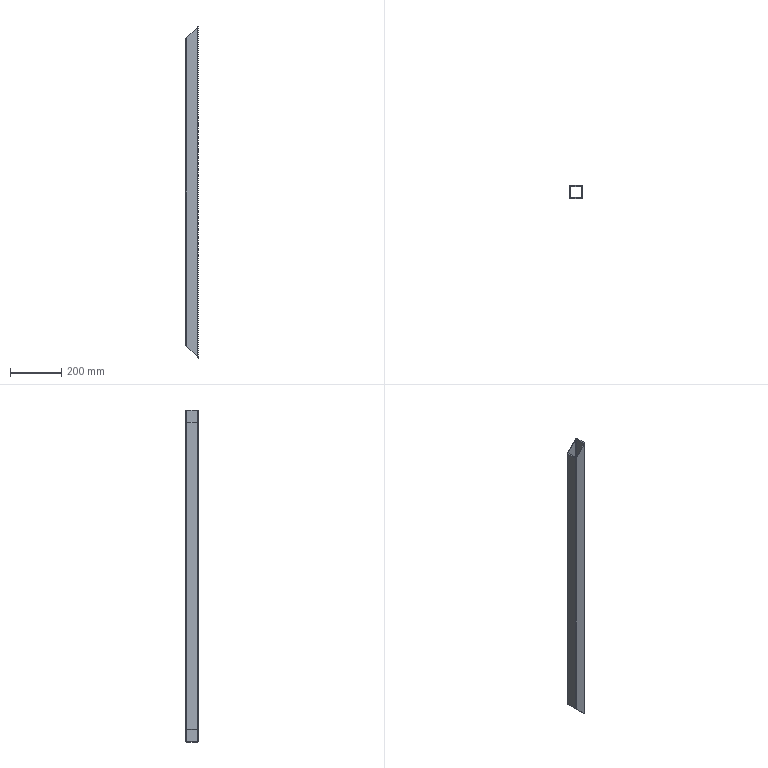Part | SolidWorks | features BaseBody 1 | 1 solid | 18 faces | box 50 x 50 x 1296 mm | volume 686700 mm3 | plane 10 | cylinder 8 | commonest cylinder face diameters 2 x4 8 x4
STEP:
#1=CARTESIAN_POINT('',(-25.,21.,598.));
#2=VERTEX_POINT('',#1);
#3=CARTESIAN_POINT('',(-25.,21.,-598.));
#4=VERTEX_POINT('',#3);
#5=CARTESIAN_POINT('',(-25.,21.,648.));
#6=DIRECTION('',(0.,0.,-1.));
#7=VECTOR('',#6,1000.);
#8=LINE('',#5,#7);
#9=EDGE_CURVE('',#2,#4,#8,.T.);
#10=ORIENTED_EDGE('',*,*,#9,.T.);
#11=CARTESIAN_POINT('',(-25.,-21.,-598.));
#12=VERTEX_POINT('',#11);
#13=CARTESIAN_POINT('',(-25.,-25.,-598.));
#14=DIRECTION('',(0.,1.,0.));
#15=VECTOR('',#14,1000.);
#16=LINE('',#13,#15);
#17=EDGE_CURVE('',#12,#4,#16,.T.);
#18=ORIENTED_EDGE('',*,*,#17,.F.);
#19=CARTESIAN_POINT('',(-25.,-21.,598.));
#20=VERTEX_POINT('',#19);
#21=CARTESIAN_POINT('',(-25.,-21.,648.));
#22=DIRECTION('',(0.,0.,-1.));
#23=VECTOR('',#22,1000.);
#24=LINE('',#21,#23);
#25=EDGE_CURVE('',#20,#12,#24,.T.);
#26=ORIENTED_EDGE('',*,*,#25,.F.);
#27=CARTESIAN_POINT('',(-25.,-25.,598.));
#28=DIRECTION('',(0.,1.,0.));
#29=VECTOR('',#28,1000.);
#30=LINE('',#27,#29);
#31=EDGE_CURVE('',#20,#2,#30,.T.);
#32=ORIENTED_EDGE('',*,*,#31,.T.);
#33=EDGE_LOOP('',(#10,#18,#26,#32));
#34=FACE_OUTER_BOUND('',#33,.T.);
#35=CARTESIAN_POINT('',(-25.,21.,648.));
#36=DIRECTION('',(1.,0.,0.));
#37=DIRECTION('',(0.,1.,0.));
#38=AXIS2_PLACEMENT_3D('',#35,#36,#37);
#39=PLANE('',#38);
#40=ADVANCED_FACE('',(#34),#39,.F.);
#41=CARTESIAN_POINT('',(-21.,25.,602.));
#42=VERTEX_POINT('',#41);
#43=CARTESIAN_POINT('',(-21.,25.,-602.));
#44=VERTEX_POINT('',#43);
#45=CARTESIAN_POINT('',(-21.,25.,648.));
#46=DIRECTION('',(0.,0.,-1.));
#47=VECTOR('',#46,1000.);
#48=LINE('',#45,#47);
#49=EDGE_CURVE('',#42,#44,#48,.T.);
#50=ORIENTED_EDGE('',*,*,#49,.T.);
#51=CARTESIAN_POINT('',(-21.,25.,-602.));
#52=CARTESIAN_POINT('',(-23.343,25.,-599.657));
#53=CARTESIAN_POINT('',(-25.,23.343,-598.));
#54=CARTESIAN_POINT('',(-25.,21.,-598.));
#55=(BOUNDED_CURVE()B_SPLINE_CURVE(3,(#51,#52,#53,#54),.UNSPECIFIED.,.F.,.F.)B_SPLINE_CURVE_WITH_KNOTS((4,4),(1.571,3.142),.UNSPECIFIED.)CURVE()GEOMETRIC_REPRESENTATION_ITEM()RATIONAL_B_SPLINE_CURVE((1.,0.8047,0.8047,1.))REPRESENTATION_ITEM(''));
#56=EDGE_CURVE('',#44,#4,#55,.T.);
#57=ORIENTED_EDGE('',*,*,#56,.T.);
#58=ORIENTED_EDGE('',*,*,#9,.F.);
#59=CARTESIAN_POINT('',(-25.,21.,598.));
#60=CARTESIAN_POINT('',(-25.,23.343,598.));
#61=CARTESIAN_POINT('',(-23.343,25.,599.657));
#62=CARTESIAN_POINT('',(-21.,25.,602.));
#63=(BOUNDED_CURVE()B_SPLINE_CURVE(3,(#59,#60,#61,#62),.UNSPECIFIED.,.F.,.F.)B_SPLINE_CURVE_WITH_KNOTS((4,4),(0.,1.571),.UNSPECIFIED.)CURVE()GEOMETRIC_REPRESENTATION_ITEM()RATIONAL_B_SPLINE_CURVE((1.,0.8047,0.8047,1.))REPRESENTATION_ITEM(''));
#64=EDGE_CURVE('',#2,#42,#63,.T.);
#65=ORIENTED_EDGE('',*,*,#64,.T.);
#66=EDGE_LOOP('',(#50,#57,#58,#65));
#67=FACE_OUTER_BOUND('',#66,.T.);
#68=CARTESIAN_POINT('',(-21.,21.,648.));
#69=DIRECTION('',(0.,0.,-1.));
#70=DIRECTION('',(-1.,0.,0.));
#71=AXIS2_PLACEMENT_3D('',#68,#69,#70);
#72=CYLINDRICAL_SURFACE('',#71,4.);
#73=ADVANCED_FACE('',(#67),#72,.T.);
#74=CARTESIAN_POINT('',(21.,25.,644.));
#75=VERTEX_POINT('',#74);
#76=CARTESIAN_POINT('',(21.,25.,-644.));
#77=VERTEX_POINT('',#76);
#78=CARTESIAN_POINT('',(21.,25.,648.));
#79=DIRECTION('',(0.,0.,-1.));
#80=VECTOR('',#79,1000.);
#81=LINE('',#78,#80);
#82=EDGE_CURVE('',#75,#77,#81,.T.);
#83=ORIENTED_EDGE('',*,*,#82,.T.);
#84=CARTESIAN_POINT('',(25.,25.,-648.));
#85=DIRECTION('',(0.7071,0.,-0.7071));
#86=VECTOR('',#85,1000.);
#87=LINE('',#84,#86);
#88=EDGE_CURVE('',#44,#77,#87,.T.);
#89=ORIENTED_EDGE('',*,*,#88,.F.);
#90=ORIENTED_EDGE('',*,*,#49,.F.);
#91=CARTESIAN_POINT('',(25.,25.,648.));
#92=DIRECTION('',(-0.7071,0.,-0.7071));
#93=VECTOR('',#92,1000.);
#94=LINE('',#91,#93);
#95=EDGE_CURVE('',#75,#42,#94,.T.);
#96=ORIENTED_EDGE('',*,*,#95,.F.);
#97=EDGE_LOOP('',(#83,#89,#90,#96));
#98=FACE_OUTER_BOUND('',#97,.T.);
#99=CARTESIAN_POINT('',(-21.,25.,648.));
#100=DIRECTION('',(0.,-1.,0.));
#101=DIRECTION('',(0.,0.,-1.));
#102=AXIS2_PLACEMENT_3D('',#99,#100,#101);
#103=PLANE('',#102);
#104=ADVANCED_FACE('',(#98),#103,.F.);
#105=CARTESIAN_POINT('',(25.,21.,648.));
#106=VERTEX_POINT('',#105);
#107=CARTESIAN_POINT('',(25.,21.,-648.));
#108=VERTEX_POINT('',#107);
#109=CARTESIAN_POINT('',(25.,21.,648.));
#110=DIRECTION('',(0.,0.,-1.));
#111=VECTOR('',#110,1000.);
#112=LINE('',#109,#111);
#113=EDGE_CURVE('',#106,#108,#112,.T.);
#114=ORIENTED_EDGE('',*,*,#113,.T.);
#115=CARTESIAN_POINT('',(25.,21.,-648.));
#116=CARTESIAN_POINT('',(25.,23.343,-648.));
#117=CARTESIAN_POINT('',(23.343,25.,-646.343));
#118=CARTESIAN_POINT('',(21.,25.,-644.));
#119=(BOUNDED_CURVE()B_SPLINE_CURVE(3,(#115,#116,#117,#118),.UNSPECIFIED.,.F.,.F.)B_SPLINE_CURVE_WITH_KNOTS((4,4),(0.,1.571),.UNSPECIFIED.)CURVE()GEOMETRIC_REPRESENTATION_ITEM()RATIONAL_B_SPLINE_CURVE((1.,0.8047,0.8047,1.))REPRESENTATION_ITEM(''));
#120=EDGE_CURVE('',#108,#77,#119,.T.);
#121=ORIENTED_EDGE('',*,*,#120,.T.);
#122=ORIENTED_EDGE('',*,*,#82,.F.);
#123=CARTESIAN_POINT('',(21.,25.,644.));
#124=CARTESIAN_POINT('',(23.343,25.,646.343));
#125=CARTESIAN_POINT('',(25.,23.343,648.));
#126=CARTESIAN_POINT('',(25.,21.,648.));
#127=(BOUNDED_CURVE()B_SPLINE_CURVE(3,(#123,#124,#125,#126),.UNSPECIFIED.,.F.,.F.)B_SPLINE_CURVE_WITH_KNOTS((4,4),(1.571,3.142),.UNSPECIFIED.)CURVE()GEOMETRIC_REPRESENTATION_ITEM()RATIONAL_B_SPLINE_CURVE((1.,0.8047,0.8047,1.))REPRESENTATION_ITEM(''));
#128=EDGE_CURVE('',#75,#106,#127,.T.);
#129=ORIENTED_EDGE('',*,*,#128,.T.);
#130=EDGE_LOOP('',(#114,#121,#122,#129));
#131=FACE_OUTER_BOUND('',#130,.T.);
#132=CARTESIAN_POINT('',(21.,21.,648.));
#133=DIRECTION('',(0.,0.,-1.));
#134=DIRECTION('',(-1.,0.,0.));
#135=AXIS2_PLACEMENT_3D('',#132,#133,#134);
#136=CYLINDRICAL_SURFACE('',#135,4.);
#137=ADVANCED_FACE('',(#131),#136,.T.);
#138=CARTESIAN_POINT('',(25.,-21.,-648.));
#139=VERTEX_POINT('',#138);
#140=CARTESIAN_POINT('',(25.,21.,-648.));
#141=DIRECTION('',(0.,1.,0.));
#142=VECTOR('',#141,1000.);
#143=LINE('',#140,#142);
#144=EDGE_CURVE('',#139,#108,#143,.T.);
#145=ORIENTED_EDGE('',*,*,#144,.T.);
#146=ORIENTED_EDGE('',*,*,#113,.F.);
#147=CARTESIAN_POINT('',(25.,-21.,648.));
#148=VERTEX_POINT('',#147);
#149=CARTESIAN_POINT('',(25.,21.,648.));
#150=DIRECTION('',(0.,1.,0.));
#151=VECTOR('',#150,1000.);
#152=LINE('',#149,#151);
#153=EDGE_CURVE('',#148,#106,#152,.T.);
#154=ORIENTED_EDGE('',*,*,#153,.F.);
#155=CARTESIAN_POINT('',(25.,-21.,648.));
#156=DIRECTION('',(0.,0.,-1.));
#157=VECTOR('',#156,1000.);
#158=LINE('',#155,#157);
#159=EDGE_CURVE('',#148,#139,#158,.T.);
#160=ORIENTED_EDGE('',*,*,#159,.T.);
#161=EDGE_LOOP('',(#145,#146,#154,#160));
#162=FACE_OUTER_BOUND('',#161,.T.);
#163=CARTESIAN_POINT('',(25.,21.,648.));
#164=DIRECTION('',(-1.,0.,0.));
#165=DIRECTION('',(0.,1.,0.));
#166=AXIS2_PLACEMENT_3D('',#163,#164,#165);
#167=PLANE('',#166);
#168=ADVANCED_FACE('',(#162),#167,.F.);
#169=CARTESIAN_POINT('',(21.,-25.,644.));
#170=VERTEX_POINT('',#169);
#171=CARTESIAN_POINT('',(21.,-25.,-644.));
#172=VERTEX_POINT('',#171);
#173=CARTESIAN_POINT('',(21.,-25.,648.));
#174=DIRECTION('',(0.,0.,-1.));
#175=VECTOR('',#174,1000.);
#176=LINE('',#173,#175);
#177=EDGE_CURVE('',#170,#172,#176,.T.);
#178=ORIENTED_EDGE('',*,*,#177,.T.);
#179=CARTESIAN_POINT('',(21.,-25.,-644.));
#180=CARTESIAN_POINT('',(23.343,-25.,-646.343));
#181=CARTESIAN_POINT('',(25.,-23.343,-648.));
#182=CARTESIAN_POINT('',(25.,-21.,-648.));
#183=(BOUNDED_CURVE()B_SPLINE_CURVE(3,(#179,#180,#181,#182),.UNSPECIFIED.,.F.,.F.)B_SPLINE_CURVE_WITH_KNOTS((4,4),(4.712,6.283),.UNSPECIFIED.)CURVE()GEOMETRIC_REPRESENTATION_ITEM()RATIONAL_B_SPLINE_CURVE((1.,0.8047,0.8047,1.))REPRESENTATION_ITEM(''));
#184=EDGE_CURVE('',#172,#139,#183,.T.);
#185=ORIENTED_EDGE('',*,*,#184,.T.);
#186=ORIENTED_EDGE('',*,*,#159,.F.);
#187=CARTESIAN_POINT('',(25.,-21.,648.));
#188=CARTESIAN_POINT('',(25.,-23.343,648.));
#189=CARTESIAN_POINT('',(23.343,-25.,646.343));
#190=CARTESIAN_POINT('',(21.,-25.,644.));
#191=(BOUNDED_CURVE()B_SPLINE_CURVE(3,(#187,#188,#189,#190),.UNSPECIFIED.,.F.,.F.)B_SPLINE_CURVE_WITH_KNOTS((4,4),(3.142,4.712),.UNSPECIFIED.)CURVE()GEOMETRIC_REPRESENTATION_ITEM()RATIONAL_B_SPLINE_CURVE((1.,0.8047,0.8047,1.))REPRESENTATION_ITEM(''));
#192=EDGE_CURVE('',#148,#170,#191,.T.);
#193=ORIENTED_EDGE('',*,*,#192,.T.);
#194=EDGE_LOOP('',(#178,#185,#186,#193));
#195=FACE_OUTER_BOUND('',#194,.T.);
#196=CARTESIAN_POINT('',(21.,-21.,648.));
#197=DIRECTION('',(0.,0.,-1.));
#198=DIRECTION('',(-1.,0.,0.));
#199=AXIS2_PLACEMENT_3D('',#196,#197,#198);
#200=CYLINDRICAL_SURFACE('',#199,4.);
#201=ADVANCED_FACE('',(#195),#200,.T.);
#202=CARTESIAN_POINT('',(-21.,-25.,602.));
#203=VERTEX_POINT('',#202);
#204=CARTESIAN_POINT('',(-21.,-25.,-602.));
#205=VERTEX_POINT('',#204);
#206=CARTESIAN_POINT('',(-21.,-25.,648.));
#207=DIRECTION('',(0.,0.,-1.));
#208=VECTOR('',#207,1000.);
#209=LINE('',#206,#208);
#210=EDGE_CURVE('',#203,#205,#209,.T.);
#211=ORIENTED_EDGE('',*,*,#210,.T.);
#212=CARTESIAN_POINT('',(25.,-25.,-648.));
#213=DIRECTION('',(0.7071,0.,-0.7071));
#214=VECTOR('',#213,1000.);
#215=LINE('',#212,#214);
#216=EDGE_CURVE('',#205,#172,#215,.T.);
#217=ORIENTED_EDGE('',*,*,#216,.T.);
#218=ORIENTED_EDGE('',*,*,#177,.F.);
#219=CARTESIAN_POINT('',(25.,-25.,648.));
#220=DIRECTION('',(-0.7071,0.,-0.7071));
#221=VECTOR('',#220,1000.);
#222=LINE('',#219,#221);
#223=EDGE_CURVE('',#170,#203,#222,.T.);
#224=ORIENTED_EDGE('',*,*,#223,.T.);
#225=EDGE_LOOP('',(#211,#217,#218,#224));
#226=FACE_OUTER_BOUND('',#225,.T.);
#227=CARTESIAN_POINT('',(-21.,-25.,648.));
#228=DIRECTION('',(0.,1.,0.));
#229=DIRECTION('',(1.,0.,0.));
#230=AXIS2_PLACEMENT_3D('',#227,#228,#229);
#231=PLANE('',#230);
#232=ADVANCED_FACE('',(#226),#231,.F.);
#233=ORIENTED_EDGE('',*,*,#25,.T.);
#234=CARTESIAN_POINT('',(-25.,-21.,-598.));
#235=CARTESIAN_POINT('',(-25.,-23.343,-598.));
#236=CARTESIAN_POINT('',(-23.343,-25.,-599.657));
#237=CARTESIAN_POINT('',(-21.,-25.,-602.));
#238=(BOUNDED_CURVE()B_SPLINE_CURVE(3,(#234,#235,#236,#237),.UNSPECIFIED.,.F.,.F.)B_SPLINE_CURVE_WITH_KNOTS((4,4),(3.142,4.712),.UNSPECIFIED.)CURVE()GEOMETRIC_REPRESENTATION_ITEM()RATIONAL_B_SPLINE_CURVE((1.,0.8047,0.8047,1.))REPRESENTATION_ITEM(''));
#239=EDGE_CURVE('',#12,#205,#238,.T.);
#240=ORIENTED_EDGE('',*,*,#239,.T.);
#241=ORIENTED_EDGE('',*,*,#210,.F.);
#242=CARTESIAN_POINT('',(-21.,-25.,602.));
#243=CARTESIAN_POINT('',(-23.343,-25.,599.657));
#244=CARTESIAN_POINT('',(-25.,-23.343,598.));
#245=CARTESIAN_POINT('',(-25.,-21.,598.));
#246=(BOUNDED_CURVE()B_SPLINE_CURVE(3,(#242,#243,#244,#245),.UNSPECIFIED.,.F.,.F.)B_SPLINE_CURVE_WITH_KNOTS((4,4),(4.712,6.283),.UNSPECIFIED.)CURVE()GEOMETRIC_REPRESENTATION_ITEM()RATIONAL_B_SPLINE_CURVE((1.,0.8047,0.8047,1.))REPRESENTATION_ITEM(''));
#247=EDGE_CURVE('',#203,#20,#246,.T.);
#248=ORIENTED_EDGE('',*,*,#247,.T.);
#249=EDGE_LOOP('',(#233,#240,#241,#248));
#250=FACE_OUTER_BOUND('',#249,.T.);
#251=CARTESIAN_POINT('',(-21.,-21.,648.));
#252=DIRECTION('',(0.,0.,-1.));
#253=DIRECTION('',(-1.,0.,0.));
#254=AXIS2_PLACEMENT_3D('',#251,#252,#253);
#255=CYLINDRICAL_SURFACE('',#254,4.);
#256=ADVANCED_FACE('',(#250),#255,.T.);
#257=CARTESIAN_POINT('',(-22.,-21.,-601.));
#258=VERTEX_POINT('',#257);
#259=CARTESIAN_POINT('',(-21.,-22.,-602.));
#260=VERTEX_POINT('',#259);
#261=CARTESIAN_POINT('',(-22.,-21.,-601.));
#262=CARTESIAN_POINT('',(-22.,-21.586,-601.));
#263=CARTESIAN_POINT('',(-21.586,-22.,-601.414));
#264=CARTESIAN_POINT('',(-21.,-22.,-602.));
#265=(BOUNDED_CURVE()B_SPLINE_CURVE(3,(#261,#262,#263,#264),.UNSPECIFIED.,.F.,.F.)B_SPLINE_CURVE_WITH_KNOTS((4,4),(3.142,4.712),.UNSPECIFIED.)CURVE()GEOMETRIC_REPRESENTATION_ITEM()RATIONAL_B_SPLINE_CURVE((1.,0.8047,0.8047,1.))REPRESENTATION_ITEM(''));
#266=EDGE_CURVE('',#258,#260,#265,.T.);
#267=ORIENTED_EDGE('',*,*,#266,.T.);
#268=CARTESIAN_POINT('',(21.,-22.,-644.));
#269=VERTEX_POINT('',#268);
#270=CARTESIAN_POINT('',(-646.,-22.,23.));
#271=DIRECTION('',(0.7071,0.,-0.7071));
#272=VECTOR('',#271,1000.);
#273=LINE('',#270,#272);
#274=EDGE_CURVE('',#260,#269,#273,.T.);
#275=ORIENTED_EDGE('',*,*,#274,.T.);
#276=CARTESIAN_POINT('',(22.,-21.,-645.));
#277=VERTEX_POINT('',#276);
#278=CARTESIAN_POINT('',(21.,-22.,-644.));
#279=CARTESIAN_POINT('',(21.586,-22.,-644.586));
#280=CARTESIAN_POINT('',(22.,-21.586,-645.));
#281=CARTESIAN_POINT('',(22.,-21.,-645.));
#282=(BOUNDED_CURVE()B_SPLINE_CURVE(3,(#278,#279,#280,#281),.UNSPECIFIED.,.F.,.F.)B_SPLINE_CURVE_WITH_KNOTS((4,4),(4.712,6.283),.UNSPECIFIED.)CURVE()GEOMETRIC_REPRESENTATION_ITEM()RATIONAL_B_SPLINE_CURVE((1.,0.8047,0.8047,1.))REPRESENTATION_ITEM(''));
#283=EDGE_CURVE('',#269,#277,#282,.T.);
#284=ORIENTED_EDGE('',*,*,#283,.T.);
#285=CARTESIAN_POINT('',(22.,21.,-645.));
#286=VERTEX_POINT('',#285);
#287=CARTESIAN_POINT('',(22.,21.,-645.));
#288=DIRECTION('',(0.,1.,0.));
#289=VECTOR('',#288,1000.);
#290=LINE('',#287,#289);
#291=EDGE_CURVE('',#277,#286,#290,.T.);
#292=ORIENTED_EDGE('',*,*,#291,.T.);
#293=CARTESIAN_POINT('',(21.,22.,-644.));
#294=VERTEX_POINT('',#293);
#295=CARTESIAN_POINT('',(22.,21.,-645.));
#296=CARTESIAN_POINT('',(22.,21.586,-645.));
#297=CARTESIAN_POINT('',(21.586,22.,-644.586));
#298=CARTESIAN_POINT('',(21.,22.,-644.));
#299=(BOUNDED_CURVE()B_SPLINE_CURVE(3,(#295,#296,#297,#298),.UNSPECIFIED.,.F.,.F.)B_SPLINE_CURVE_WITH_KNOTS((4,4),(0.,1.571),.UNSPECIFIED.)CURVE()GEOMETRIC_REPRESENTATION_ITEM()RATIONAL_B_SPLINE_CURVE((1.,0.8047,0.8047,1.))REPRESENTATION_ITEM(''));
#300=EDGE_CURVE('',#286,#294,#299,.T.);
#301=ORIENTED_EDGE('',*,*,#300,.T.);
#302=CARTESIAN_POINT('',(-21.,22.,-602.));
#303=VERTEX_POINT('',#302);
#304=CARTESIAN_POINT('',(-646.,22.,23.));
#305=DIRECTION('',(-0.7071,0.,0.7071));
#306=VECTOR('',#305,1000.);
#307=LINE('',#304,#306);
#308=EDGE_CURVE('',#294,#303,#307,.T.);
#309=ORIENTED_EDGE('',*,*,#308,.T.);
#310=CARTESIAN_POINT('',(-22.,21.,-601.));
#311=VERTEX_POINT('',#310);
#312=CARTESIAN_POINT('',(-21.,22.,-602.));
#313=CARTESIAN_POINT('',(-21.586,22.,-601.414));
#314=CARTESIAN_POINT('',(-22.,21.586,-601.));
#315=CARTESIAN_POINT('',(-22.,21.,-601.));
#316=(BOUNDED_CURVE()B_SPLINE_CURVE(3,(#312,#313,#314,#315),.UNSPECIFIED.,.F.,.F.)B_SPLINE_CURVE_WITH_KNOTS((4,4),(1.571,3.142),.UNSPECIFIED.)CURVE()GEOMETRIC_REPRESENTATION_ITEM()RATIONAL_B_SPLINE_CURVE((1.,0.8047,0.8047,1.))REPRESENTATION_ITEM(''));
#317=EDGE_CURVE('',#303,#311,#316,.T.);
#318=ORIENTED_EDGE('',*,*,#317,.T.);
#319=CARTESIAN_POINT('',(-22.,21.,-601.));
#320=DIRECTION('',(0.,-1.,0.));
#321=VECTOR('',#320,1000.);
#322=LINE('',#319,#321);
#323=EDGE_CURVE('',#311,#258,#322,.T.);
#324=ORIENTED_EDGE('',*,*,#323,.T.);
#325=EDGE_LOOP('',(#267,#275,#284,#292,#301,#309,#318,#324));
#326=FACE_BOUND('',#325,.T.);
#327=ORIENTED_EDGE('',*,*,#17,.T.);
#328=ORIENTED_EDGE('',*,*,#56,.F.);
#329=ORIENTED_EDGE('',*,*,#88,.T.);
#330=ORIENTED_EDGE('',*,*,#120,.F.);
#331=ORIENTED_EDGE('',*,*,#144,.F.);
#332=ORIENTED_EDGE('',*,*,#184,.F.);
#333=ORIENTED_EDGE('',*,*,#216,.F.);
#334=ORIENTED_EDGE('',*,*,#239,.F.);
#335=EDGE_LOOP('',(#327,#328,#329,#330,#331,#332,#333,#334));
#336=FACE_OUTER_BOUND('',#335,.T.);
#337=CARTESIAN_POINT('',(25.,-25.,-648.));
#338=DIRECTION('',(0.7071,0.,0.7071));
#339=DIRECTION('',(0.,-1.,0.));
#340=AXIS2_PLACEMENT_3D('',#337,#338,#339);
#341=PLANE('',#340);
#342=ADVANCED_FACE('',(#326,#336),#341,.F.);
#343=CARTESIAN_POINT('',(-21.,-22.,602.));
#344=VERTEX_POINT('',#343);
#345=CARTESIAN_POINT('',(-22.,-21.,601.));
#346=VERTEX_POINT('',#345);
#347=CARTESIAN_POINT('',(-21.,-22.,602.));
#348=CARTESIAN_POINT('',(-21.586,-22.,601.414));
#349=CARTESIAN_POINT('',(-22.,-21.586,601.));
#350=CARTESIAN_POINT('',(-22.,-21.,601.));
#351=(BOUNDED_CURVE()B_SPLINE_CURVE(3,(#347,#348,#349,#350),.UNSPECIFIED.,.F.,.F.)B_SPLINE_CURVE_WITH_KNOTS((4,4),(4.712,6.283),.UNSPECIFIED.)CURVE()GEOMETRIC_REPRESENTATION_ITEM()RATIONAL_B_SPLINE_CURVE((1.,0.8047,0.8047,1.))REPRESENTATION_ITEM(''));
#352=EDGE_CURVE('',#344,#346,#351,.T.);
#353=ORIENTED_EDGE('',*,*,#352,.T.);
#354=CARTESIAN_POINT('',(-22.,21.,601.));
#355=VERTEX_POINT('',#354);
#356=CARTESIAN_POINT('',(-22.,21.,601.));
#357=DIRECTION('',(0.,1.,0.));
#358=VECTOR('',#357,1000.);
#359=LINE('',#356,#358);
#360=EDGE_CURVE('',#346,#355,#359,.T.);
#361=ORIENTED_EDGE('',*,*,#360,.T.);
#362=CARTESIAN_POINT('',(-21.,22.,602.));
#363=VERTEX_POINT('',#362);
#364=CARTESIAN_POINT('',(-22.,21.,601.));
#365=CARTESIAN_POINT('',(-22.,21.586,601.));
#366=CARTESIAN_POINT('',(-21.586,22.,601.414));
#367=CARTESIAN_POINT('',(-21.,22.,602.));
#368=(BOUNDED_CURVE()B_SPLINE_CURVE(3,(#364,#365,#366,#367),.UNSPECIFIED.,.F.,.F.)B_SPLINE_CURVE_WITH_KNOTS((4,4),(0.,1.571),.UNSPECIFIED.)CURVE()GEOMETRIC_REPRESENTATION_ITEM()RATIONAL_B_SPLINE_CURVE((1.,0.8047,0.8047,1.))REPRESENTATION_ITEM(''));
#369=EDGE_CURVE('',#355,#363,#368,.T.);
#370=ORIENTED_EDGE('',*,*,#369,.T.);
#371=CARTESIAN_POINT('',(21.,22.,644.));
#372=VERTEX_POINT('',#371);
#373=CARTESIAN_POINT('',(2.,22.,625.));
#374=DIRECTION('',(0.7071,0.,0.7071));
#375=VECTOR('',#374,1000.);
#376=LINE('',#373,#375);
#377=EDGE_CURVE('',#363,#372,#376,.T.);
#378=ORIENTED_EDGE('',*,*,#377,.T.);
#379=CARTESIAN_POINT('',(22.,21.,645.));
#380=VERTEX_POINT('',#379);
#381=CARTESIAN_POINT('',(21.,22.,644.));
#382=CARTESIAN_POINT('',(21.586,22.,644.586));
#383=CARTESIAN_POINT('',(22.,21.586,645.));
#384=CARTESIAN_POINT('',(22.,21.,645.));
#385=(BOUNDED_CURVE()B_SPLINE_CURVE(3,(#381,#382,#383,#384),.UNSPECIFIED.,.F.,.F.)B_SPLINE_CURVE_WITH_KNOTS((4,4),(1.571,3.142),.UNSPECIFIED.)CURVE()GEOMETRIC_REPRESENTATION_ITEM()RATIONAL_B_SPLINE_CURVE((1.,0.8047,0.8047,1.))REPRESENTATION_ITEM(''));
#386=EDGE_CURVE('',#372,#380,#385,.T.);
#387=ORIENTED_EDGE('',*,*,#386,.T.);
#388=CARTESIAN_POINT('',(22.,-21.,645.));
#389=VERTEX_POINT('',#388);
#390=CARTESIAN_POINT('',(22.,21.,645.));
#391=DIRECTION('',(0.,-1.,0.));
#392=VECTOR('',#391,1000.);
#393=LINE('',#390,#392);
#394=EDGE_CURVE('',#380,#389,#393,.T.);
#395=ORIENTED_EDGE('',*,*,#394,.T.);
#396=CARTESIAN_POINT('',(21.,-22.,644.));
#397=VERTEX_POINT('',#396);
#398=CARTESIAN_POINT('',(22.,-21.,645.));
#399=CARTESIAN_POINT('',(22.,-21.586,645.));
#400=CARTESIAN_POINT('',(21.586,-22.,644.586));
#401=CARTESIAN_POINT('',(21.,-22.,644.));
#402=(BOUNDED_CURVE()B_SPLINE_CURVE(3,(#398,#399,#400,#401),.UNSPECIFIED.,.F.,.F.)B_SPLINE_CURVE_WITH_KNOTS((4,4),(3.142,4.712),.UNSPECIFIED.)CURVE()GEOMETRIC_REPRESENTATION_ITEM()RATIONAL_B_SPLINE_CURVE((1.,0.8047,0.8047,1.))REPRESENTATION_ITEM(''));
#403=EDGE_CURVE('',#389,#397,#402,.T.);
#404=ORIENTED_EDGE('',*,*,#403,.T.);
#405=CARTESIAN_POINT('',(2.,-22.,625.));
#406=DIRECTION('',(-0.7071,0.,-0.7071));
#407=VECTOR('',#406,1000.);
#408=LINE('',#405,#407);
#409=EDGE_CURVE('',#397,#344,#408,.T.);
#410=ORIENTED_EDGE('',*,*,#409,.T.);
#411=EDGE_LOOP('',(#353,#361,#370,#378,#387,#395,#404,#410));
#412=FACE_BOUND('',#411,.T.);
#413=ORIENTED_EDGE('',*,*,#223,.F.);
#414=ORIENTED_EDGE('',*,*,#192,.F.);
#415=ORIENTED_EDGE('',*,*,#153,.T.);
#416=ORIENTED_EDGE('',*,*,#128,.F.);
#417=ORIENTED_EDGE('',*,*,#95,.T.);
#418=ORIENTED_EDGE('',*,*,#64,.F.);
#419=ORIENTED_EDGE('',*,*,#31,.F.);
#420=ORIENTED_EDGE('',*,*,#247,.F.);
#421=EDGE_LOOP('',(#413,#414,#415,#416,#417,#418,#419,#420));
#422=FACE_OUTER_BOUND('',#421,.T.);
#423=CARTESIAN_POINT('',(25.,-25.,648.));
#424=DIRECTION('',(0.7071,0.,-0.7071));
#425=DIRECTION('',(0.,-1.,0.));
#426=AXIS2_PLACEMENT_3D('',#423,#424,#425);
#427=PLANE('',#426);
#428=ADVANCED_FACE('',(#412,#422),#427,.F.);
#429=ORIENTED_EDGE('',*,*,#266,.F.);
#430=CARTESIAN_POINT('',(-22.,-21.,648.));
#431=DIRECTION('',(0.,0.,-1.));
#432=VECTOR('',#431,1000.);
#433=LINE('',#430,#432);
#434=EDGE_CURVE('',#346,#258,#433,.T.);
#435=ORIENTED_EDGE('',*,*,#434,.F.);
#436=ORIENTED_EDGE('',*,*,#352,.F.);
#437=CARTESIAN_POINT('',(-21.,-22.,648.));
#438=DIRECTION('',(0.,0.,-1.));
#439=VECTOR('',#438,1000.);
#440=LINE('',#437,#439);
#441=EDGE_CURVE('',#344,#260,#440,.T.);
#442=ORIENTED_EDGE('',*,*,#441,.T.);
#443=EDGE_LOOP('',(#429,#435,#436,#442));
#444=FACE_OUTER_BOUND('',#443,.T.);
#445=CARTESIAN_POINT('',(-21.,-21.,648.));
#446=DIRECTION('',(0.,0.,-1.));
#447=DIRECTION('',(-1.,0.,0.));
#448=AXIS2_PLACEMENT_3D('',#445,#446,#447);
#449=CYLINDRICAL_SURFACE('',#448,1.);
#450=ADVANCED_FACE('',(#444),#449,.F.);
#451=ORIENTED_EDGE('',*,*,#274,.F.);
#452=ORIENTED_EDGE('',*,*,#441,.F.);
#453=ORIENTED_EDGE('',*,*,#409,.F.);
#454=CARTESIAN_POINT('',(21.,-22.,648.));
#455=DIRECTION('',(0.,0.,-1.));
#456=VECTOR('',#455,1000.);
#457=LINE('',#454,#456);
#458=EDGE_CURVE('',#397,#269,#457,.T.);
#459=ORIENTED_EDGE('',*,*,#458,.T.);
#460=EDGE_LOOP('',(#451,#452,#453,#459));
#461=FACE_OUTER_BOUND('',#460,.T.);
#462=CARTESIAN_POINT('',(-21.,-22.,648.));
#463=DIRECTION('',(0.,1.,0.));
#464=DIRECTION('',(1.,0.,0.));
#465=AXIS2_PLACEMENT_3D('',#462,#463,#464);
#466=PLANE('',#465);
#467=ADVANCED_FACE('',(#461),#466,.T.);
#468=ORIENTED_EDGE('',*,*,#283,.F.);
#469=ORIENTED_EDGE('',*,*,#458,.F.);
#470=ORIENTED_EDGE('',*,*,#403,.F.);
#471=CARTESIAN_POINT('',(22.,-21.,648.));
#472=DIRECTION('',(0.,0.,-1.));
#473=VECTOR('',#472,1000.);
#474=LINE('',#471,#473);
#475=EDGE_CURVE('',#389,#277,#474,.T.);
#476=ORIENTED_EDGE('',*,*,#475,.T.);
#477=EDGE_LOOP('',(#468,#469,#470,#476));
#478=FACE_OUTER_BOUND('',#477,.T.);
#479=CARTESIAN_POINT('',(21.,-21.,648.));
#480=DIRECTION('',(0.,0.,-1.));
#481=DIRECTION('',(-1.,0.,0.));
#482=AXIS2_PLACEMENT_3D('',#479,#480,#481);
#483=CYLINDRICAL_SURFACE('',#482,1.);
#484=ADVANCED_FACE('',(#478),#483,.F.);
#485=ORIENTED_EDGE('',*,*,#291,.F.);
#486=ORIENTED_EDGE('',*,*,#475,.F.);
#487=ORIENTED_EDGE('',*,*,#394,.F.);
#488=CARTESIAN_POINT('',(22.,21.,648.));
#489=DIRECTION('',(0.,0.,-1.));
#490=VECTOR('',#489,1000.);
#491=LINE('',#488,#490);
#492=EDGE_CURVE('',#380,#286,#491,.T.);
#493=ORIENTED_EDGE('',*,*,#492,.T.);
#494=EDGE_LOOP('',(#485,#486,#487,#493));
#495=FACE_OUTER_BOUND('',#494,.T.);
#496=CARTESIAN_POINT('',(22.,21.,648.));
#497=DIRECTION('',(-1.,0.,0.));
#498=DIRECTION('',(0.,1.,0.));
#499=AXIS2_PLACEMENT_3D('',#496,#497,#498);
#500=PLANE('',#499);
#501=ADVANCED_FACE('',(#495),#500,.T.);
#502=ORIENTED_EDGE('',*,*,#300,.F.);
#503=ORIENTED_EDGE('',*,*,#492,.F.);
#504=ORIENTED_EDGE('',*,*,#386,.F.);
#505=CARTESIAN_POINT('',(21.,22.,648.));
#506=DIRECTION('',(0.,0.,-1.));
#507=VECTOR('',#506,1000.);
#508=LINE('',#505,#507);
#509=EDGE_CURVE('',#372,#294,#508,.T.);
#510=ORIENTED_EDGE('',*,*,#509,.T.);
#511=EDGE_LOOP('',(#502,#503,#504,#510));
#512=FACE_OUTER_BOUND('',#511,.T.);
#513=CARTESIAN_POINT('',(21.,21.,648.));
#514=DIRECTION('',(0.,0.,-1.));
#515=DIRECTION('',(-1.,0.,0.));
#516=AXIS2_PLACEMENT_3D('',#513,#514,#515);
#517=CYLINDRICAL_SURFACE('',#516,1.);
#518=ADVANCED_FACE('',(#512),#517,.F.);
#519=ORIENTED_EDGE('',*,*,#308,.F.);
#520=ORIENTED_EDGE('',*,*,#509,.F.);
#521=ORIENTED_EDGE('',*,*,#377,.F.);
#522=CARTESIAN_POINT('',(-21.,22.,648.));
#523=DIRECTION('',(0.,0.,-1.));
#524=VECTOR('',#523,1000.);
#525=LINE('',#522,#524);
#526=EDGE_CURVE('',#363,#303,#525,.T.);
#527=ORIENTED_EDGE('',*,*,#526,.T.);
#528=EDGE_LOOP('',(#519,#520,#521,#527));
#529=FACE_OUTER_BOUND('',#528,.T.);
#530=CARTESIAN_POINT('',(-21.,22.,648.));
#531=DIRECTION('',(0.,-1.,0.));
#532=DIRECTION('',(0.,0.,-1.));
#533=AXIS2_PLACEMENT_3D('',#530,#531,#532);
#534=PLANE('',#533);
#535=ADVANCED_FACE('',(#529),#534,.T.);
#536=ORIENTED_EDGE('',*,*,#317,.F.);
#537=ORIENTED_EDGE('',*,*,#526,.F.);
#538=ORIENTED_EDGE('',*,*,#369,.F.);
#539=CARTESIAN_POINT('',(-22.,21.,648.));
#540=DIRECTION('',(0.,0.,-1.));
#541=VECTOR('',#540,1000.);
#542=LINE('',#539,#541);
#543=EDGE_CURVE('',#355,#311,#542,.T.);
#544=ORIENTED_EDGE('',*,*,#543,.T.);
#545=EDGE_LOOP('',(#536,#537,#538,#544));
#546=FACE_OUTER_BOUND('',#545,.T.);
#547=CARTESIAN_POINT('',(-21.,21.,648.));
#548=DIRECTION('',(0.,0.,-1.));
#549=DIRECTION('',(-1.,0.,0.));
#550=AXIS2_PLACEMENT_3D('',#547,#548,#549);
#551=CYLINDRICAL_SURFACE('',#550,1.);
#552=ADVANCED_FACE('',(#546),#551,.F.);
#553=ORIENTED_EDGE('',*,*,#323,.F.);
#554=ORIENTED_EDGE('',*,*,#543,.F.);
#555=ORIENTED_EDGE('',*,*,#360,.F.);
#556=ORIENTED_EDGE('',*,*,#434,.T.);
#557=EDGE_LOOP('',(#553,#554,#555,#556));
#558=FACE_OUTER_BOUND('',#557,.T.);
#559=CARTESIAN_POINT('',(-22.,21.,648.));
#560=DIRECTION('',(1.,0.,0.));
#561=DIRECTION('',(0.,1.,0.));
#562=AXIS2_PLACEMENT_3D('',#559,#560,#561);
#563=PLANE('',#562);
#564=ADVANCED_FACE('',(#558),#563,.T.);
#565=CLOSED_SHELL('',(#40,#73,#104,#137,#168,#201,#232,#256,#342,#428,#450,#467,#484,#501,#518,#535,#552,#564));
#566=MANIFOLD_SOLID_BREP('',#565);
#567=CARTESIAN_POINT('',(0.,0.,0.));
#568=DIRECTION('',(0.,0.,1.));
#569=DIRECTION('',(1.,0.,0.));
#570=AXIS2_PLACEMENT_3D('',#567,#568,#569);
#571=(LENGTH_UNIT()NAMED_UNIT(*)SI_UNIT(.MILLI.,.METRE.));
#572=UNCERTAINTY_MEASURE_WITH_UNIT(LENGTH_MEASURE(0.00001),#571,'','');
#573=(NAMED_UNIT(*)PLANE_ANGLE_UNIT()SI_UNIT($,.RADIAN.));
#574=(NAMED_UNIT(*)SI_UNIT($,.STERADIAN.)SOLID_ANGLE_UNIT());
#575=(GEOMETRIC_REPRESENTATION_CONTEXT(3)GLOBAL_UNCERTAINTY_ASSIGNED_CONTEXT((#572))GLOBAL_UNIT_ASSIGNED_CONTEXT((#571,#573,#574))REPRESENTATION_CONTEXT('',''));
#576=ADVANCED_BREP_SHAPE_REPRESENTATION('',(#566,#570),#575);